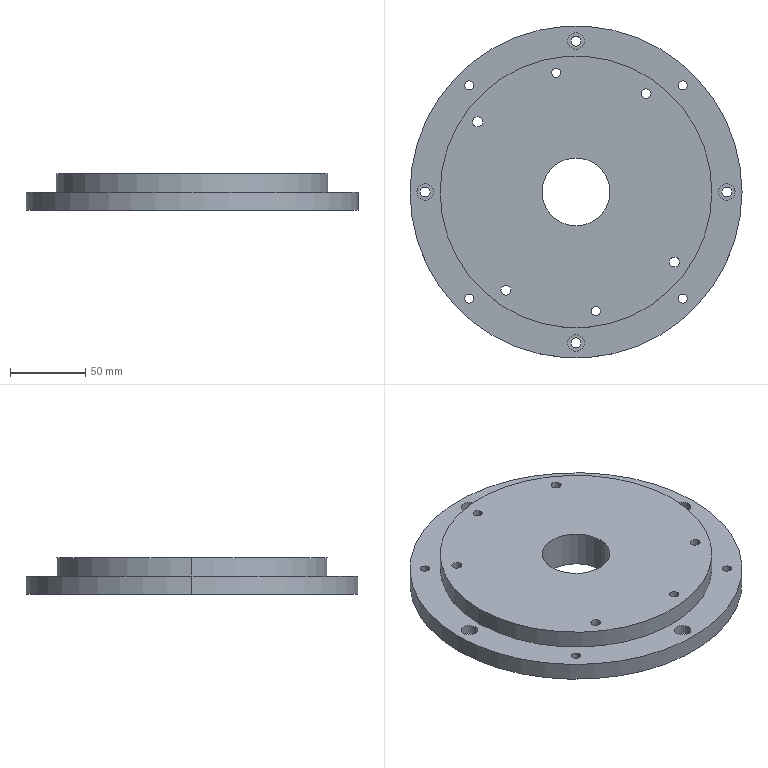Part | STEP file | 11-FG-Z00811 | 1 solid | 61 faces | box 220 x 220 x 24 mm | volume 712597 mm3 | cylinder 50 | plane 11 | commonest cylinder face diameters 6.6 x16 11 x16 6 x12 45 x2 180 x2 220 x2